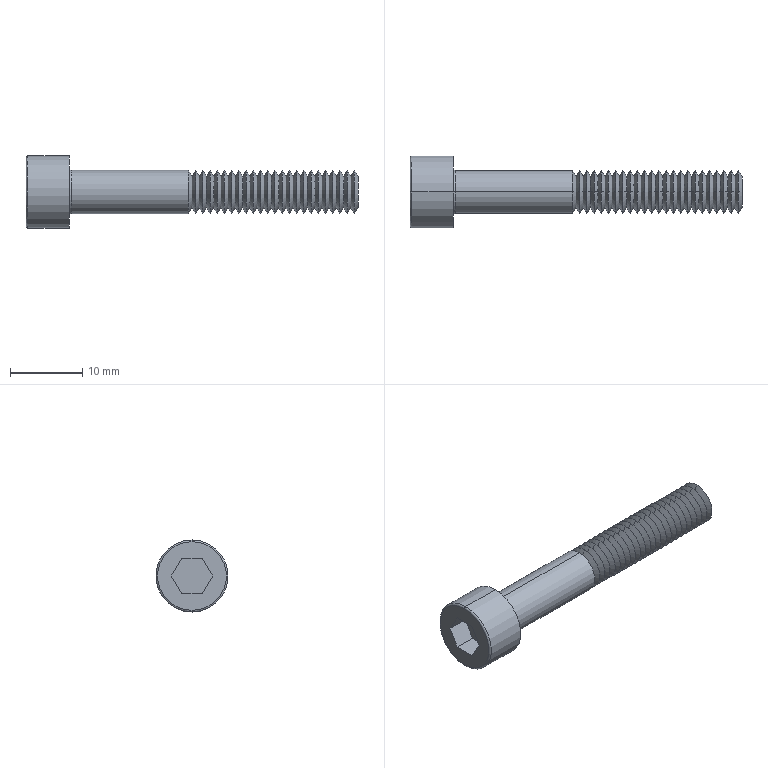Part | SolidWorks | features BlendCut 1, Cut 1, Fillet 1, LPattern 1, RevCut 1, Revolution 1 | 1 solid | 112 faces | box 46 x 10 x 10 mm | volume 1365 mm3 | cone 94 | plane 10 | cylinder 4 | torus 4 | commonest cylinder face diameters 6 x2 10 x2